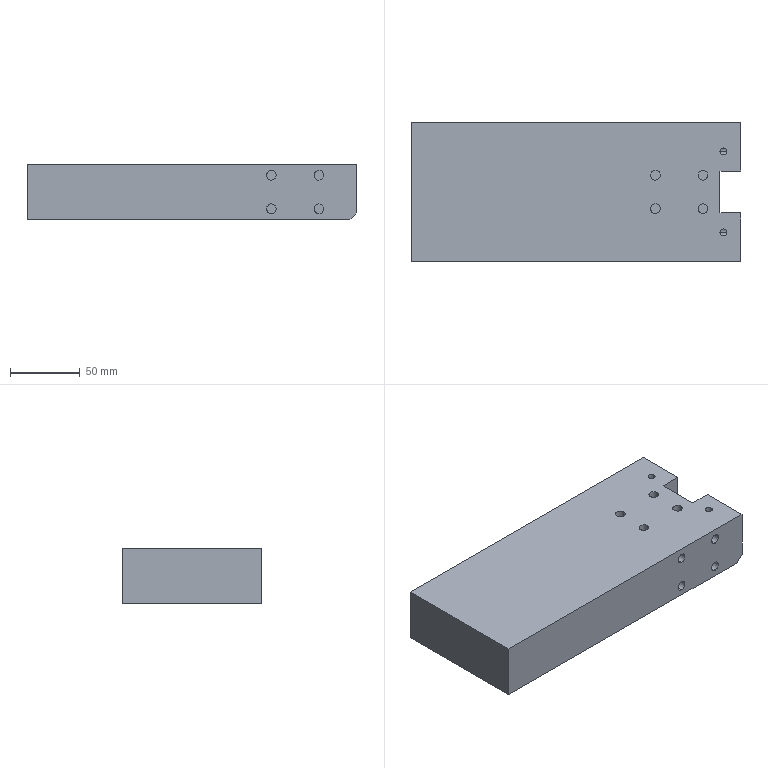Part | STEP file | Positioning_id2066_x_t | 1 solid | 64 faces | box 236.25 x 100 x 40 mm | volume 918195 mm3 | cylinder 36 | plane 28 | commonest cylinder face diameters 7 x24 5 x4 10 x4 17 x4